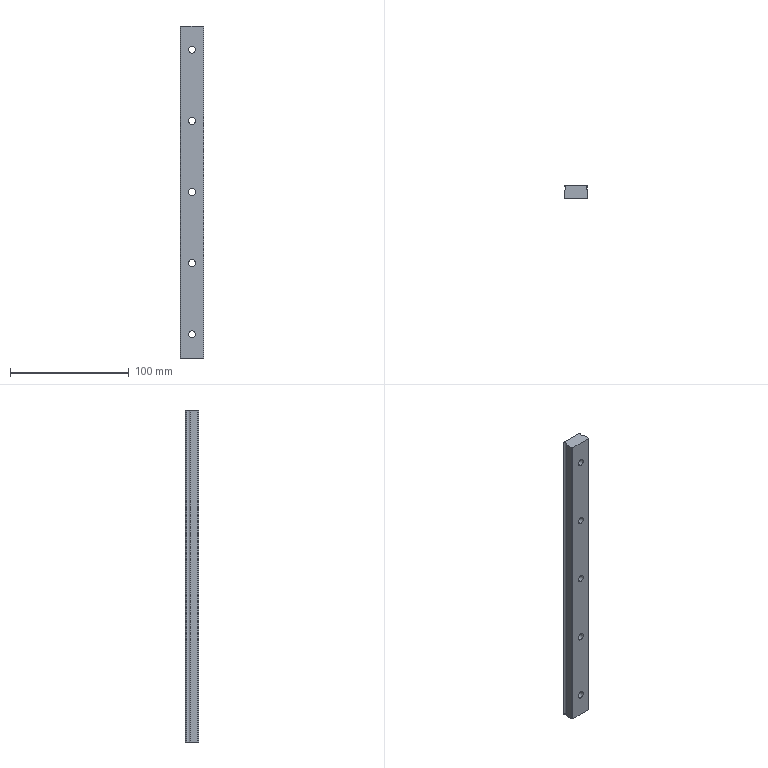Part | STEP file | r_SEBZ20_280 | 1 solid | 40 faces | box 20 x 11 x 280 mm | volume 56779 mm3 | cylinder 23 | plane 17 | commonest cylinder face diameters 6 x10 9.5 x10 3.529 x3